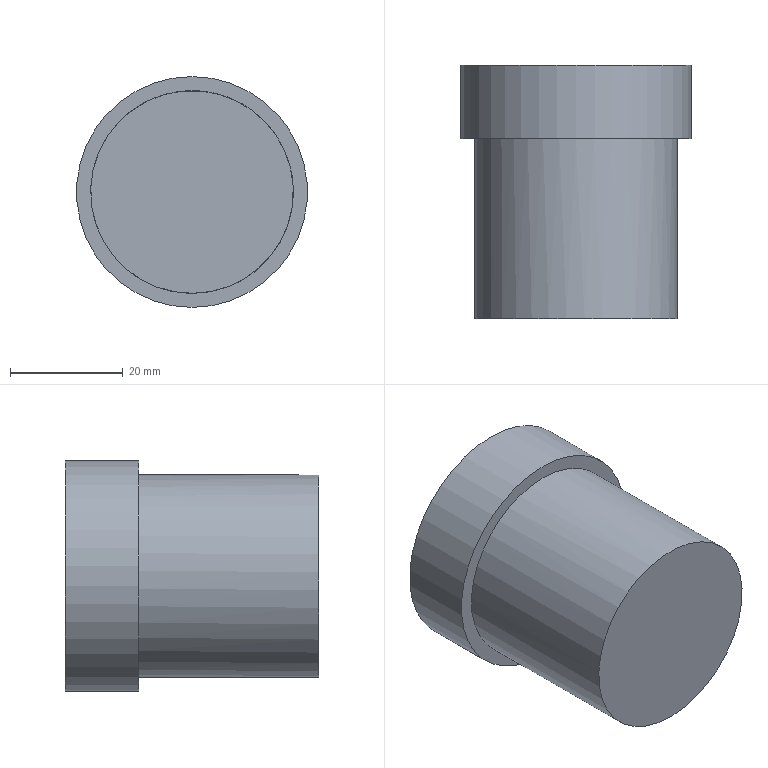Part | NX | features solid 2 | 1 solid | 5 faces | box 41 x 45 x 41 mm | volume 49735 mm3 | plane 3 | cylinder 2 | commonest cylinder face diameters 36 x1 41 x1
STEP:
#1=CARTESIAN_POINT('',(495.,762.,118.));
#2=VERTEX_POINT('',#1);
#3=CARTESIAN_POINT('',(495.,762.,100.));
#4=DIRECTION('',(0.,1.,0.));
#5=DIRECTION('',(0.,0.,1.));
#6=AXIS2_PLACEMENT_3D('',#3,#4,#5);
#7=CIRCLE('',#6,18.);
#8=EDGE_CURVE('',#2,#2,#7,.T.);
#9=ORIENTED_EDGE('',*,*,#8,.T.);
#10=EDGE_LOOP('',(#9));
#11=FACE_BOUND('',#10,.T.);
#12=CARTESIAN_POINT('',(512.162,762.,88.788));
#13=VERTEX_POINT('',#12);
#14=CARTESIAN_POINT('',(495.,762.,100.));
#15=DIRECTION('',(0.,-1.,0.));
#16=DIRECTION('',(0.8372,0.,-0.5469));
#17=AXIS2_PLACEMENT_3D('',#14,#15,#16);
#18=CIRCLE('',#17,20.5);
#19=EDGE_CURVE('',#13,#13,#18,.T.);
#20=ORIENTED_EDGE('',*,*,#19,.T.);
#21=EDGE_LOOP('',(#20));
#22=FACE_BOUND('',#21,.T.);
#23=CARTESIAN_POINT('',(495.,762.,100.));
#24=DIRECTION('',(0.,-1.,0.));
#25=DIRECTION('',(-0.8372,0.,0.5469));
#26=AXIS2_PLACEMENT_3D('',#23,#24,#25);
#27=PLANE('',#26);
#28=ADVANCED_FACE('',(#11,#22),#27,.T.);
#29=CARTESIAN_POINT('',(477.838,775.,111.212));
#30=VERTEX_POINT('',#29);
#31=CARTESIAN_POINT('',(495.,775.,100.));
#32=DIRECTION('',(0.,1.,0.));
#33=DIRECTION('',(-0.8372,0.,0.5469));
#34=AXIS2_PLACEMENT_3D('',#31,#32,#33);
#35=CIRCLE('',#34,20.5);
#36=EDGE_CURVE('',#30,#30,#35,.T.);
#37=ORIENTED_EDGE('',*,*,#36,.T.);
#38=EDGE_LOOP('',(#37));
#39=FACE_BOUND('',#38,.T.);
#40=CARTESIAN_POINT('',(495.,775.,100.));
#41=DIRECTION('',(0.,1.,0.));
#42=DIRECTION('',(0.8372,0.,-0.5469));
#43=AXIS2_PLACEMENT_3D('',#40,#41,#42);
#44=PLANE('',#43);
#45=ADVANCED_FACE('',(#39),#44,.T.);
#46=ORIENTED_EDGE('',*,*,#19,.F.);
#47=EDGE_LOOP('',(#46));
#48=FACE_BOUND('',#47,.T.);
#49=ORIENTED_EDGE('',*,*,#36,.F.);
#50=EDGE_LOOP('',(#49));
#51=FACE_BOUND('',#50,.T.);
#52=CARTESIAN_POINT('',(495.,775.,100.));
#53=DIRECTION('',(0.,-1.,0.));
#54=DIRECTION('',(-0.8372,0.,0.5469));
#55=AXIS2_PLACEMENT_3D('',#52,#53,#54);
#56=CYLINDRICAL_SURFACE('',#55,20.5);
#57=ADVANCED_FACE('',(#48,#51),#56,.T.);
#58=CARTESIAN_POINT('',(479.931,730.,109.845));
#59=VERTEX_POINT('',#58);
#60=CARTESIAN_POINT('',(495.,730.,100.));
#61=DIRECTION('',(0.,1.,0.));
#62=DIRECTION('',(-0.8372,0.,0.5469));
#63=AXIS2_PLACEMENT_3D('',#60,#61,#62);
#64=CIRCLE('',#63,18.);
#65=EDGE_CURVE('',#59,#59,#64,.T.);
#66=ORIENTED_EDGE('',*,*,#65,.F.);
#67=EDGE_LOOP('',(#66));
#68=FACE_BOUND('',#67,.T.);
#69=CARTESIAN_POINT('',(495.,730.,100.));
#70=DIRECTION('',(0.,-1.,0.));
#71=DIRECTION('',(-0.8372,0.,0.5469));
#72=AXIS2_PLACEMENT_3D('',#69,#70,#71);
#73=PLANE('',#72);
#74=ADVANCED_FACE('',(#68),#73,.T.);
#75=ORIENTED_EDGE('',*,*,#65,.T.);
#76=EDGE_LOOP('',(#75));
#77=FACE_BOUND('',#76,.T.);
#78=ORIENTED_EDGE('',*,*,#8,.F.);
#79=EDGE_LOOP('',(#78));
#80=FACE_BOUND('',#79,.T.);
#81=CARTESIAN_POINT('',(495.,762.,100.));
#82=DIRECTION('',(0.,-1.,0.));
#83=DIRECTION('',(-0.8372,0.,0.5469));
#84=AXIS2_PLACEMENT_3D('',#81,#82,#83);
#85=CYLINDRICAL_SURFACE('',#84,18.);
#86=ADVANCED_FACE('',(#77,#80),#85,.T.);
#87=CLOSED_SHELL('',(#28,#45,#57,#74,#86));
#88=MANIFOLD_SOLID_BREP('',#87);
#89=(LENGTH_UNIT()NAMED_UNIT(*)SI_UNIT(.MILLI.,.METRE.));
#90=UNCERTAINTY_MEASURE_WITH_UNIT(LENGTH_MEASURE(0.00001),#89,'','');
#91=(NAMED_UNIT(*)PLANE_ANGLE_UNIT()SI_UNIT($,.RADIAN.));
#92=(NAMED_UNIT(*)SI_UNIT($,.STERADIAN.)SOLID_ANGLE_UNIT());
#93=(GEOMETRIC_REPRESENTATION_CONTEXT(3)GLOBAL_UNCERTAINTY_ASSIGNED_CONTEXT((#90))GLOBAL_UNIT_ASSIGNED_CONTEXT((#89,#91,#92))REPRESENTATION_CONTEXT('',''));
#94=ADVANCED_BREP_SHAPE_REPRESENTATION('',(#88),#93);